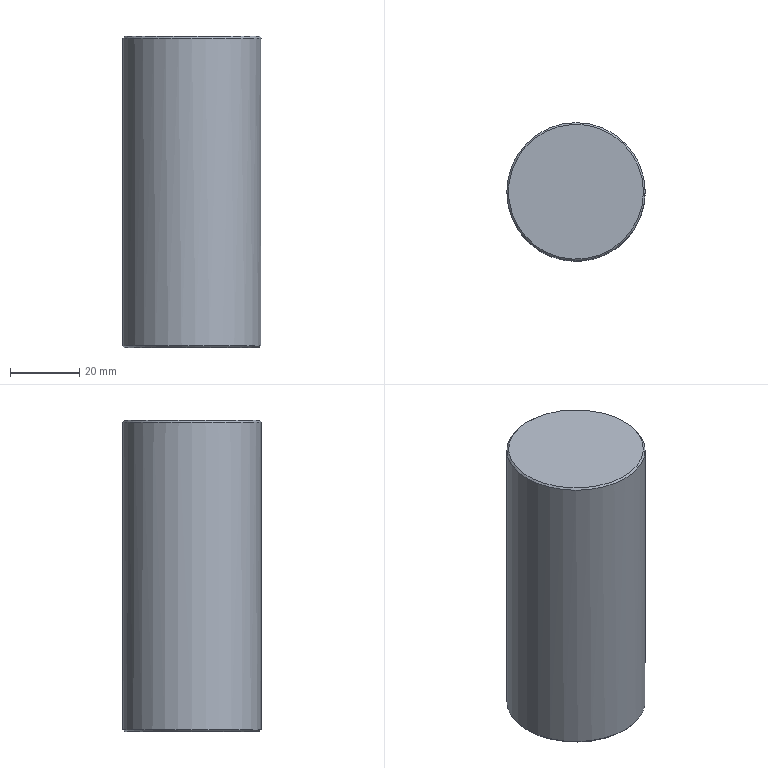Part | STEP file | lll_id110_x_t | 1 solid | 9 faces | box 40 x 40 x 90 mm | volume 111990 mm3 | cylinder 4 | cone 3 | plane 2 | commonest cylinder face diameters 10 x2 8.5 x1 40 x1
STEP:
#1=CARTESIAN_POINT('',(-19.5,-100.,-165.5));
#2=VERTEX_POINT('',#1);
#3=CARTESIAN_POINT('',(0.,-100.,-165.5));
#4=DIRECTION('',(0.,0.,-1.));
#5=DIRECTION('',(-1.,0.,0.));
#6=AXIS2_PLACEMENT_3D('',#3,#4,#5);
#7=CIRCLE('',#6,19.5);
#8=EDGE_CURVE('',#2,#2,#7,.T.);
#9=ORIENTED_EDGE('',*,*,#8,.T.);
#10=EDGE_LOOP('',(#9));
#11=FACE_BOUND('',#10,.T.);
#12=CARTESIAN_POINT('',(5.,-100.,-165.5));
#13=VERTEX_POINT('',#12);
#14=CARTESIAN_POINT('',(0.,-95.,-165.5));
#15=VERTEX_POINT('',#14);
#16=CARTESIAN_POINT('',(0.,-100.,-165.5));
#17=DIRECTION('',(0.,0.,-1.));
#18=DIRECTION('',(-1.,0.,0.));
#19=AXIS2_PLACEMENT_3D('',#16,#17,#18);
#20=CIRCLE('',#19,5.);
#21=EDGE_CURVE('',#13,#15,#20,.T.);
#22=ORIENTED_EDGE('',*,*,#21,.F.);
#23=CARTESIAN_POINT('',(0.,-100.,-165.5));
#24=DIRECTION('',(0.,0.,1.));
#25=DIRECTION('',(1.,0.,0.));
#26=AXIS2_PLACEMENT_3D('',#23,#24,#25);
#27=CIRCLE('',#26,5.);
#28=EDGE_CURVE('',#15,#13,#27,.T.);
#29=ORIENTED_EDGE('',*,*,#28,.F.);
#30=EDGE_LOOP('',(#22,#29));
#31=FACE_BOUND('',#30,.T.);
#32=CARTESIAN_POINT('',(4.25,-100.,-165.5));
#33=VERTEX_POINT('',#32);
#34=CARTESIAN_POINT('',(0.,-100.,-165.5));
#35=DIRECTION('',(0.,0.,1.));
#36=DIRECTION('',(1.,0.,0.));
#37=AXIS2_PLACEMENT_3D('',#34,#35,#36);
#38=CIRCLE('',#37,4.25);
#39=EDGE_CURVE('',#33,#33,#38,.T.);
#40=ORIENTED_EDGE('',*,*,#39,.T.);
#41=EDGE_LOOP('',(#40));
#42=FACE_BOUND('',#41,.T.);
#43=CARTESIAN_POINT('',(0.,-100.,-165.5));
#44=DIRECTION('',(0.,0.,-1.));
#45=DIRECTION('',(-1.,0.,0.));
#46=AXIS2_PLACEMENT_3D('',#43,#44,#45);
#47=PLANE('',#46);
#48=ADVANCED_FACE('',(#11,#31,#42),#47,.T.);
#49=CARTESIAN_POINT('',(19.5,-100.,-75.5));
#50=VERTEX_POINT('',#49);
#51=CARTESIAN_POINT('',(0.,-100.,-75.5));
#52=DIRECTION('',(0.,0.,1.));
#53=DIRECTION('',(1.,0.,0.));
#54=AXIS2_PLACEMENT_3D('',#51,#52,#53);
#55=CIRCLE('',#54,19.5);
#56=EDGE_CURVE('',#50,#50,#55,.T.);
#57=ORIENTED_EDGE('',*,*,#56,.T.);
#58=EDGE_LOOP('',(#57));
#59=FACE_OUTER_BOUND('',#58,.T.);
#60=CARTESIAN_POINT('',(0.,-100.,-75.5));
#61=DIRECTION('',(0.,0.,1.));
#62=DIRECTION('',(1.,0.,0.));
#63=AXIS2_PLACEMENT_3D('',#60,#61,#62);
#64=PLANE('',#63);
#65=ADVANCED_FACE('',(#59),#64,.T.);
#66=CARTESIAN_POINT('',(-20.,-100.,-165.));
#67=VERTEX_POINT('',#66);
#68=CARTESIAN_POINT('',(0.,-100.,-165.));
#69=DIRECTION('',(0.,0.,1.));
#70=DIRECTION('',(-1.,0.,0.));
#71=AXIS2_PLACEMENT_3D('',#68,#69,#70);
#72=CIRCLE('',#71,20.);
#73=EDGE_CURVE('',#67,#67,#72,.T.);
#74=ORIENTED_EDGE('',*,*,#73,.T.);
#75=EDGE_LOOP('',(#74));
#76=FACE_BOUND('',#75,.T.);
#77=CARTESIAN_POINT('',(20.,-100.,-76.));
#78=VERTEX_POINT('',#77);
#79=CARTESIAN_POINT('',(0.,-100.,-76.));
#80=DIRECTION('',(0.,0.,-1.));
#81=DIRECTION('',(1.,0.,0.));
#82=AXIS2_PLACEMENT_3D('',#79,#80,#81);
#83=CIRCLE('',#82,20.);
#84=EDGE_CURVE('',#78,#78,#83,.T.);
#85=ORIENTED_EDGE('',*,*,#84,.T.);
#86=EDGE_LOOP('',(#85));
#87=FACE_BOUND('',#86,.T.);
#88=CARTESIAN_POINT('',(0.,-100.,-75.5));
#89=DIRECTION('',(0.,0.,-1.));
#90=DIRECTION('',(-1.,0.,0.));
#91=AXIS2_PLACEMENT_3D('',#88,#89,#90);
#92=CYLINDRICAL_SURFACE('',#91,20.);
#93=ADVANCED_FACE('',(#76,#87),#92,.T.);
#94=CARTESIAN_POINT('',(4.25,-100.,-147.5));
#95=VERTEX_POINT('',#94);
#96=CARTESIAN_POINT('',(0.,-100.,-147.5));
#97=DIRECTION('',(0.,0.,1.));
#98=DIRECTION('',(1.,0.,0.));
#99=AXIS2_PLACEMENT_3D('',#96,#97,#98);
#100=CIRCLE('',#99,4.25);
#101=EDGE_CURVE('',#95,#95,#100,.T.);
#102=ORIENTED_EDGE('',*,*,#101,.T.);
#103=EDGE_LOOP('',(#102));
#104=FACE_BOUND('',#103,.T.);
#105=ORIENTED_EDGE('',*,*,#39,.F.);
#106=EDGE_LOOP('',(#105));
#107=FACE_BOUND('',#106,.T.);
#108=CARTESIAN_POINT('',(0.,-100.,-165.5));
#109=DIRECTION('',(0.,0.,1.));
#110=DIRECTION('',(1.,0.,0.));
#111=AXIS2_PLACEMENT_3D('',#108,#109,#110);
#112=CYLINDRICAL_SURFACE('',#111,4.25);
#113=ADVANCED_FACE('',(#104,#107),#112,.F.);
#114=ORIENTED_EDGE('',*,*,#101,.F.);
#115=EDGE_LOOP('',(#114));
#116=FACE_BOUND('',#115,.T.);
#117=CARTESIAN_POINT('',(0.,-100.,-144.61));
#118=VERTEX_POINT('',#117);
#119=VERTEX_LOOP('',#118);
#120=FACE_BOUND('',#119,.T.);
#121=CARTESIAN_POINT('',(0.,-100.,-144.61));
#122=DIRECTION('',(0.,0.,-1.));
#123=DIRECTION('',(-1.,0.,0.));
#124=AXIS2_PLACEMENT_3D('',#121,#122,#123);
#125=CONICAL_SURFACE('',#124,0.,55.784);
#126=ADVANCED_FACE('',(#116,#120),#125,.F.);
#127=ORIENTED_EDGE('',*,*,#21,.T.);
#128=CARTESIAN_POINT('',(0.,-95.,-150.5));
#129=VERTEX_POINT('',#128);
#130=CARTESIAN_POINT('',(0.,-95.,-165.5));
#131=CARTESIAN_POINT('',(0.,-95.,-160.5));
#132=CARTESIAN_POINT('',(0.,-95.,-155.5));
#133=CARTESIAN_POINT('',(0.,-95.,-150.5));
#134=B_SPLINE_CURVE_WITH_KNOTS('',3,(#130,#131,#132,#133),.UNSPECIFIED.,.F.,.F.,(4,4),(0.,1.),.UNSPECIFIED.);
#135=EDGE_CURVE('',#15,#129,#134,.T.);
#136=ORIENTED_EDGE('',*,*,#135,.T.);
#137=CARTESIAN_POINT('',(5.,-100.,-150.5));
#138=VERTEX_POINT('',#137);
#139=CARTESIAN_POINT('',(0.,-95.,-150.5));
#140=CARTESIAN_POINT('',(-1.963,-95.,-150.5));
#141=CARTESIAN_POINT('',(-3.868,-96.273,-150.5));
#142=CARTESIAN_POINT('',(-5.371,-99.901,-150.5));
#143=CARTESIAN_POINT('',(-4.924,-102.147,-150.5));
#144=CARTESIAN_POINT('',(-2.147,-104.924,-150.5));
#145=CARTESIAN_POINT('',(0.09938,-105.371,-150.5));
#146=CARTESIAN_POINT('',(3.727,-103.868,-150.5));
#147=CARTESIAN_POINT('',(5.,-101.963,-150.5));
#148=CARTESIAN_POINT('',(5.,-100.,-150.5));
#149=B_SPLINE_CURVE_WITH_KNOTS('',3,(#139,#140,#141,#142,#143,#144,#145,#146,#147,#148),.UNSPECIFIED.,.F.,.F.,(4,2,2,2,4),(0.,0.25,0.5,0.75,1.),.UNSPECIFIED.);
#150=EDGE_CURVE('',#129,#138,#149,.T.);
#151=ORIENTED_EDGE('',*,*,#150,.T.);
#152=CARTESIAN_POINT('',(5.,-100.,-150.5));
#153=CARTESIAN_POINT('',(5.,-100.,-155.5));
#154=CARTESIAN_POINT('',(5.,-100.,-160.5));
#155=CARTESIAN_POINT('',(5.,-100.,-165.5));
#156=B_SPLINE_CURVE_WITH_KNOTS('',3,(#152,#153,#154,#155),.UNSPECIFIED.,.F.,.F.,(4,4),(0.,1.),.UNSPECIFIED.);
#157=EDGE_CURVE('',#138,#13,#156,.T.);
#158=ORIENTED_EDGE('',*,*,#157,.T.);
#159=EDGE_LOOP('',(#127,#136,#151,#158));
#160=FACE_OUTER_BOUND('',#159,.T.);
#161=CARTESIAN_POINT('',(0.,-100.,-166.5));
#162=DIRECTION('',(0.,0.,1.));
#163=DIRECTION('',(1.,0.,0.));
#164=AXIS2_PLACEMENT_3D('',#161,#162,#163);
#165=CYLINDRICAL_SURFACE('',#164,5.);
#166=ADVANCED_FACE('',(#160),#165,.F.);
#167=ORIENTED_EDGE('',*,*,#150,.F.);
#168=ORIENTED_EDGE('',*,*,#135,.F.);
#169=ORIENTED_EDGE('',*,*,#28,.T.);
#170=ORIENTED_EDGE('',*,*,#157,.F.);
#171=EDGE_LOOP('',(#167,#168,#169,#170));
#172=FACE_OUTER_BOUND('',#171,.T.);
#173=CARTESIAN_POINT('',(0.,-100.,-165.5));
#174=DIRECTION('',(0.,0.,1.));
#175=DIRECTION('',(1.,0.,0.));
#176=AXIS2_PLACEMENT_3D('',#173,#174,#175);
#177=CYLINDRICAL_SURFACE('',#176,5.);
#178=ADVANCED_FACE('',(#172),#177,.T.);
#179=ORIENTED_EDGE('',*,*,#8,.F.);
#180=EDGE_LOOP('',(#179));
#181=FACE_BOUND('',#180,.T.);
#182=ORIENTED_EDGE('',*,*,#73,.F.);
#183=EDGE_LOOP('',(#182));
#184=FACE_BOUND('',#183,.T.);
#185=CARTESIAN_POINT('',(0.,-100.,-165.));
#186=DIRECTION('',(0.,0.,1.));
#187=DIRECTION('',(1.,0.,0.));
#188=AXIS2_PLACEMENT_3D('',#185,#186,#187);
#189=CONICAL_SURFACE('',#188,20.,45.);
#190=ADVANCED_FACE('',(#181,#184),#189,.T.);
#191=ORIENTED_EDGE('',*,*,#56,.F.);
#192=EDGE_LOOP('',(#191));
#193=FACE_BOUND('',#192,.T.);
#194=ORIENTED_EDGE('',*,*,#84,.F.);
#195=EDGE_LOOP('',(#194));
#196=FACE_BOUND('',#195,.T.);
#197=CARTESIAN_POINT('',(0.,-100.,-76.));
#198=DIRECTION('',(0.,0.,-1.));
#199=DIRECTION('',(-1.,0.,0.));
#200=AXIS2_PLACEMENT_3D('',#197,#198,#199);
#201=CONICAL_SURFACE('',#200,20.,45.);
#202=ADVANCED_FACE('',(#193,#196),#201,.T.);
#203=CLOSED_SHELL('',(#48,#65,#93,#113,#126,#166,#178,#190,#202));
#204=MANIFOLD_SOLID_BREP('',#203);
#205=(LENGTH_UNIT()NAMED_UNIT(*)SI_UNIT(.MILLI.,.METRE.));
#206=UNCERTAINTY_MEASURE_WITH_UNIT(LENGTH_MEASURE(0.0508),#205,'','');
#207=(NAMED_UNIT(*)PLANE_ANGLE_UNIT()SI_UNIT($,.RADIAN.));
#208=PLANE_ANGLE_MEASURE_WITH_UNIT(PLANE_ANGLE_MEASURE(0.01745),#207);
#209=DIMENSIONAL_EXPONENTS(0.,0.,0.,0.,0.,0.,0.);
#210=(CONVERSION_BASED_UNIT('DEGREE',#208)NAMED_UNIT(#209)PLANE_ANGLE_UNIT());
#211=(NAMED_UNIT(*)SI_UNIT($,.STERADIAN.)SOLID_ANGLE_UNIT());
#212=(GEOMETRIC_REPRESENTATION_CONTEXT(3)GLOBAL_UNCERTAINTY_ASSIGNED_CONTEXT((#206))GLOBAL_UNIT_ASSIGNED_CONTEXT((#205,#210,#211))REPRESENTATION_CONTEXT('',''));
#213=ADVANCED_BREP_SHAPE_REPRESENTATION('',(#204),#212);